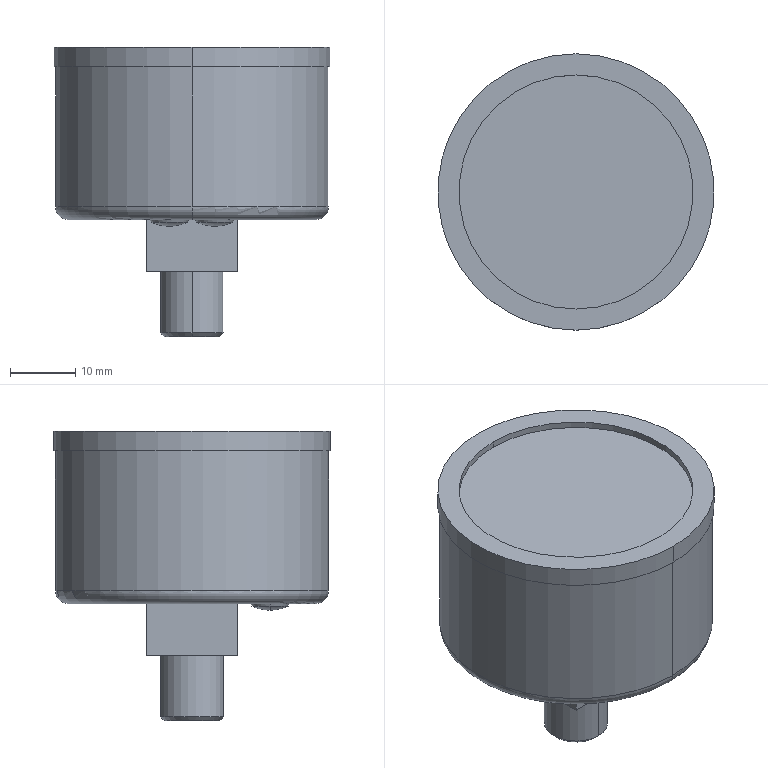Part | STEP file | G46-10-01-SRB | 1 solid | 30 faces | box 42.5 x 42.5 x 44.5 mm | volume 38027 mm3 | plane 10 | cylinder 8 | cone 6 | other 4 | torus 2 | commonest cylinder face diameters 9.728 x2 36 x2 42 x2 42.5 x2